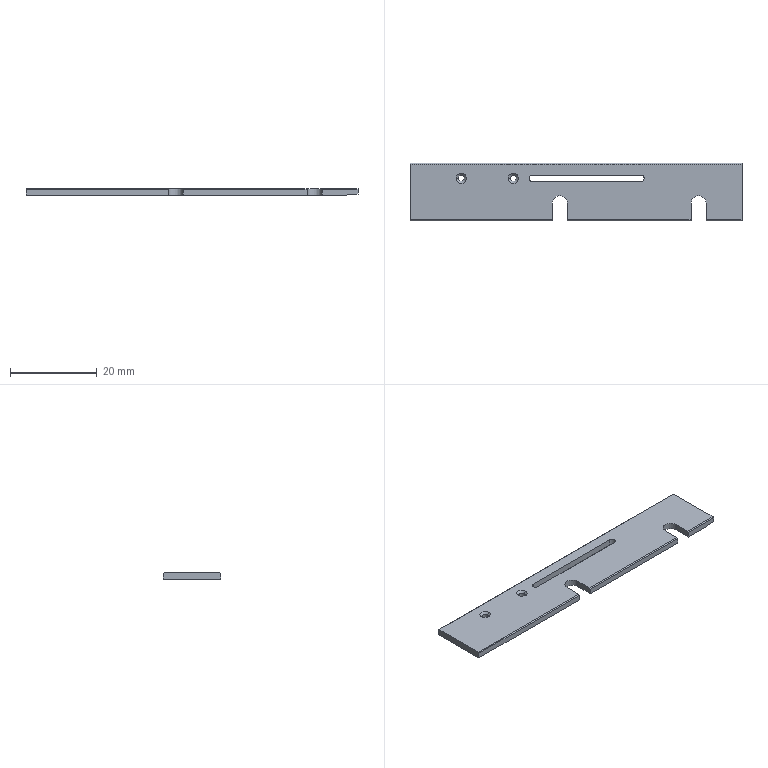Part | NX | 1 solid | 32 faces | box 76.5 x 13.2 x 1.5 mm | volume 1385 mm3 | plane 19 | cylinder 9 | cone 4 | commonest cylinder face diameters 1.4 x4 1.5 x3 3.5 x2
STEP:
#1=CARTESIAN_POINT('',(30.05,-3.5,0.75));
#2=VERTEX_POINT('',#1);
#3=CARTESIAN_POINT('',(30.05,-7.3,0.75));
#4=VERTEX_POINT('',#3);
#5=CARTESIAN_POINT('',(30.05,0.,0.75));
#6=DIRECTION('',(0.,-1.,0.));
#7=VECTOR('',#6,1000.);
#8=LINE('',#5,#7);
#9=EDGE_CURVE('',#2,#4,#8,.T.);
#10=ORIENTED_EDGE('',*,*,#9,.T.);
#11=CARTESIAN_POINT('',(38.3,-7.3,0.75));
#12=VERTEX_POINT('',#11);
#13=CARTESIAN_POINT('',(0.,-7.3,0.75));
#14=DIRECTION('',(-1.,0.,0.));
#15=VECTOR('',#14,1000.);
#16=LINE('',#13,#15);
#17=EDGE_CURVE('',#12,#4,#16,.T.);
#18=ORIENTED_EDGE('',*,*,#17,.F.);
#19=CARTESIAN_POINT('',(38.3,5.5,0.75));
#20=VERTEX_POINT('',#19);
#21=CARTESIAN_POINT('',(38.3,0.,0.75));
#22=DIRECTION('',(0.,-1.,0.));
#23=VECTOR('',#22,1000.);
#24=LINE('',#21,#23);
#25=EDGE_CURVE('',#20,#12,#24,.T.);
#26=ORIENTED_EDGE('',*,*,#25,.F.);
#27=CARTESIAN_POINT('',(-38.2,5.5,0.75));
#28=VERTEX_POINT('',#27);
#29=CARTESIAN_POINT('',(0.,5.5,0.75));
#30=DIRECTION('',(1.,0.,0.));
#31=VECTOR('',#30,1000.);
#32=LINE('',#29,#31);
#33=EDGE_CURVE('',#28,#20,#32,.T.);
#34=ORIENTED_EDGE('',*,*,#33,.F.);
#35=CARTESIAN_POINT('',(-38.2,-7.3,0.75));
#36=VERTEX_POINT('',#35);
#37=CARTESIAN_POINT('',(-38.2,0.,0.75));
#38=DIRECTION('',(0.,1.,0.));
#39=VECTOR('',#38,1000.);
#40=LINE('',#37,#39);
#41=EDGE_CURVE('',#36,#28,#40,.T.);
#42=ORIENTED_EDGE('',*,*,#41,.F.);
#43=CARTESIAN_POINT('',(-5.45,-7.3,0.75));
#44=VERTEX_POINT('',#43);
#45=CARTESIAN_POINT('',(0.,-7.3,0.75));
#46=DIRECTION('',(-1.,0.,0.));
#47=VECTOR('',#46,1000.);
#48=LINE('',#45,#47);
#49=EDGE_CURVE('',#44,#36,#48,.T.);
#50=ORIENTED_EDGE('',*,*,#49,.F.);
#51=CARTESIAN_POINT('',(-5.45,-3.5,0.75));
#52=VERTEX_POINT('',#51);
#53=CARTESIAN_POINT('',(-5.45,0.,0.75));
#54=DIRECTION('',(0.,1.,0.));
#55=VECTOR('',#54,1000.);
#56=LINE('',#53,#55);
#57=EDGE_CURVE('',#44,#52,#56,.T.);
#58=ORIENTED_EDGE('',*,*,#57,.T.);
#59=CARTESIAN_POINT('',(-1.95,-3.5,0.75));
#60=VERTEX_POINT('',#59);
#61=CARTESIAN_POINT('',(-3.7,-3.5,0.75));
#62=DIRECTION('',(0.,0.,-1.));
#63=DIRECTION('',(-1.,0.,0.));
#64=AXIS2_PLACEMENT_3D('',#61,#62,#63);
#65=CIRCLE('',#64,1.75);
#66=EDGE_CURVE('',#52,#60,#65,.T.);
#67=ORIENTED_EDGE('',*,*,#66,.T.);
#68=CARTESIAN_POINT('',(-1.95,-7.3,0.75));
#69=VERTEX_POINT('',#68);
#70=CARTESIAN_POINT('',(-1.95,0.,0.75));
#71=DIRECTION('',(0.,-1.,0.));
#72=VECTOR('',#71,1000.);
#73=LINE('',#70,#72);
#74=EDGE_CURVE('',#60,#69,#73,.T.);
#75=ORIENTED_EDGE('',*,*,#74,.T.);
#76=CARTESIAN_POINT('',(26.55,-7.3,0.75));
#77=VERTEX_POINT('',#76);
#78=CARTESIAN_POINT('',(0.,-7.3,0.75));
#79=DIRECTION('',(-1.,0.,0.));
#80=VECTOR('',#79,1000.);
#81=LINE('',#78,#80);
#82=EDGE_CURVE('',#77,#69,#81,.T.);
#83=ORIENTED_EDGE('',*,*,#82,.F.);
#84=CARTESIAN_POINT('',(26.55,-3.5,0.75));
#85=VERTEX_POINT('',#84);
#86=CARTESIAN_POINT('',(26.55,0.,0.75));
#87=DIRECTION('',(0.,1.,0.));
#88=VECTOR('',#87,1000.);
#89=LINE('',#86,#88);
#90=EDGE_CURVE('',#77,#85,#89,.T.);
#91=ORIENTED_EDGE('',*,*,#90,.T.);
#92=CARTESIAN_POINT('',(28.3,-3.5,0.75));
#93=DIRECTION('',(0.,0.,-1.));
#94=DIRECTION('',(-1.,0.,0.));
#95=AXIS2_PLACEMENT_3D('',#92,#93,#94);
#96=CIRCLE('',#95,1.75);
#97=EDGE_CURVE('',#85,#2,#96,.T.);
#98=ORIENTED_EDGE('',*,*,#97,.T.);
#99=EDGE_LOOP('',(#10,#18,#26,#34,#42,#50,#58,#67,#75,#83,#91,#98));
#100=FACE_BOUND('',#99,.T.);
#101=CARTESIAN_POINT('',(15.,1.5,0.75));
#102=VERTEX_POINT('',#101);
#103=CARTESIAN_POINT('',(15.,3.,0.75));
#104=VERTEX_POINT('',#103);
#105=CARTESIAN_POINT('',(15.,2.25,0.75));
#106=DIRECTION('',(0.,0.,1.));
#107=DIRECTION('',(-1.,0.,0.));
#108=AXIS2_PLACEMENT_3D('',#105,#106,#107);
#109=CIRCLE('',#108,0.75);
#110=EDGE_CURVE('',#102,#104,#109,.T.);
#111=ORIENTED_EDGE('',*,*,#110,.F.);
#112=CARTESIAN_POINT('',(-10.,1.5,0.75));
#113=VERTEX_POINT('',#112);
#114=CARTESIAN_POINT('',(0.,1.5,0.75));
#115=DIRECTION('',(-1.,0.,0.));
#116=VECTOR('',#115,1000.);
#117=LINE('',#114,#116);
#118=EDGE_CURVE('',#102,#113,#117,.T.);
#119=ORIENTED_EDGE('',*,*,#118,.T.);
#120=CARTESIAN_POINT('',(-10.75,2.25,0.75));
#121=VERTEX_POINT('',#120);
#122=CARTESIAN_POINT('',(-10.,2.25,0.75));
#123=DIRECTION('',(0.,0.,1.));
#124=DIRECTION('',(-1.,0.,0.));
#125=AXIS2_PLACEMENT_3D('',#122,#123,#124);
#126=CIRCLE('',#125,0.75);
#127=EDGE_CURVE('',#121,#113,#126,.T.);
#128=ORIENTED_EDGE('',*,*,#127,.F.);
#129=CARTESIAN_POINT('',(-10.,3.,0.75));
#130=VERTEX_POINT('',#129);
#131=CARTESIAN_POINT('',(-10.,2.25,0.75));
#132=DIRECTION('',(0.,0.,1.));
#133=DIRECTION('',(-1.,0.,0.));
#134=AXIS2_PLACEMENT_3D('',#131,#132,#133);
#135=CIRCLE('',#134,0.75);
#136=EDGE_CURVE('',#130,#121,#135,.T.);
#137=ORIENTED_EDGE('',*,*,#136,.F.);
#138=CARTESIAN_POINT('',(0.,3.,0.75));
#139=DIRECTION('',(1.,0.,0.));
#140=VECTOR('',#139,1000.);
#141=LINE('',#138,#140);
#142=EDGE_CURVE('',#130,#104,#141,.T.);
#143=ORIENTED_EDGE('',*,*,#142,.T.);
#144=EDGE_LOOP('',(#111,#119,#128,#137,#143));
#145=FACE_BOUND('',#144,.T.);
#146=CARTESIAN_POINT('',(-15.6,2.25,0.75));
#147=VERTEX_POINT('',#146);
#148=CARTESIAN_POINT('',(-13.2,2.25,0.75));
#149=VERTEX_POINT('',#148);
#150=CARTESIAN_POINT('',(-14.4,2.25,0.75));
#151=DIRECTION('',(0.,0.,1.));
#152=DIRECTION('',(1.,0.,0.));
#153=AXIS2_PLACEMENT_3D('',#150,#151,#152);
#154=CIRCLE('',#153,1.2);
#155=EDGE_CURVE('',#147,#149,#154,.T.);
#156=ORIENTED_EDGE('',*,*,#155,.F.);
#157=CARTESIAN_POINT('',(-14.4,2.25,0.75));
#158=DIRECTION('',(0.,0.,1.));
#159=DIRECTION('',(1.,0.,0.));
#160=AXIS2_PLACEMENT_3D('',#157,#158,#159);
#161=CIRCLE('',#160,1.2);
#162=EDGE_CURVE('',#149,#147,#161,.T.);
#163=ORIENTED_EDGE('',*,*,#162,.F.);
#164=EDGE_LOOP('',(#156,#163));
#165=FACE_BOUND('',#164,.T.);
#166=CARTESIAN_POINT('',(-25.2,2.25,0.75));
#167=VERTEX_POINT('',#166);
#168=CARTESIAN_POINT('',(-27.6,2.25,0.75));
#169=VERTEX_POINT('',#168);
#170=CARTESIAN_POINT('',(-26.4,2.25,0.75));
#171=DIRECTION('',(0.,0.,1.));
#172=DIRECTION('',(1.,0.,0.));
#173=AXIS2_PLACEMENT_3D('',#170,#171,#172);
#174=CIRCLE('',#173,1.2);
#175=EDGE_CURVE('',#167,#169,#174,.T.);
#176=ORIENTED_EDGE('',*,*,#175,.F.);
#177=CARTESIAN_POINT('',(-26.4,2.25,0.75));
#178=DIRECTION('',(0.,0.,1.));
#179=DIRECTION('',(1.,0.,0.));
#180=AXIS2_PLACEMENT_3D('',#177,#178,#179);
#181=CIRCLE('',#180,1.2);
#182=EDGE_CURVE('',#169,#167,#181,.T.);
#183=ORIENTED_EDGE('',*,*,#182,.F.);
#184=EDGE_LOOP('',(#176,#183));
#185=FACE_BOUND('',#184,.T.);
#186=CARTESIAN_POINT('',(0.,0.,0.75));
#187=DIRECTION('',(0.,0.,1.));
#188=DIRECTION('',(1.,0.,0.));
#189=AXIS2_PLACEMENT_3D('',#186,#187,#188);
#190=PLANE('',#189);
#191=ADVANCED_FACE('',(#100,#145,#165,#185),#190,.T.);
#192=CARTESIAN_POINT('',(30.05,-3.5,-0.75));
#193=VERTEX_POINT('',#192);
#194=CARTESIAN_POINT('',(30.05,-7.5,-0.75));
#195=VERTEX_POINT('',#194);
#196=CARTESIAN_POINT('',(30.05,0.,-0.75));
#197=DIRECTION('',(0.,-1.,0.));
#198=VECTOR('',#197,1000.);
#199=LINE('',#196,#198);
#200=EDGE_CURVE('',#193,#195,#199,.T.);
#201=ORIENTED_EDGE('',*,*,#200,.T.);
#202=CARTESIAN_POINT('',(30.05,-7.5,0.55));
#203=VERTEX_POINT('',#202);
#204=CARTESIAN_POINT('',(30.05,-7.5,0.75));
#205=DIRECTION('',(0.,0.,-1.));
#206=VECTOR('',#205,1000.);
#207=LINE('',#204,#206);
#208=EDGE_CURVE('',#203,#195,#207,.T.);
#209=ORIENTED_EDGE('',*,*,#208,.F.);
#210=CARTESIAN_POINT('',(30.05,0.,8.05));
#211=DIRECTION('',(0.,0.7071,0.7071));
#212=VECTOR('',#211,1000.);
#213=LINE('',#210,#212);
#214=EDGE_CURVE('',#203,#4,#213,.T.);
#215=ORIENTED_EDGE('',*,*,#214,.T.);
#216=ORIENTED_EDGE('',*,*,#9,.F.);
#217=CARTESIAN_POINT('',(30.05,-3.5,0.75));
#218=DIRECTION('',(0.,0.,-1.));
#219=VECTOR('',#218,1000.);
#220=LINE('',#217,#219);
#221=EDGE_CURVE('',#2,#193,#220,.T.);
#222=ORIENTED_EDGE('',*,*,#221,.T.);
#223=EDGE_LOOP('',(#201,#209,#215,#216,#222));
#224=FACE_BOUND('',#223,.T.);
#225=CARTESIAN_POINT('',(30.05,-7.5,0.75));
#226=DIRECTION('',(1.,0.,0.));
#227=DIRECTION('',(0.,1.,0.));
#228=AXIS2_PLACEMENT_3D('',#225,#226,#227);
#229=PLANE('',#228);
#230=ADVANCED_FACE('',(#224),#229,.F.);
#231=ORIENTED_EDGE('',*,*,#221,.F.);
#232=ORIENTED_EDGE('',*,*,#97,.F.);
#233=CARTESIAN_POINT('',(26.55,-3.5,-0.75));
#234=VERTEX_POINT('',#233);
#235=CARTESIAN_POINT('',(26.55,-3.5,0.75));
#236=DIRECTION('',(0.,0.,-1.));
#237=VECTOR('',#236,1000.);
#238=LINE('',#235,#237);
#239=EDGE_CURVE('',#85,#234,#238,.T.);
#240=ORIENTED_EDGE('',*,*,#239,.T.);
#241=CARTESIAN_POINT('',(28.3,-3.5,-0.75));
#242=DIRECTION('',(0.,0.,-1.));
#243=DIRECTION('',(-1.,0.,0.));
#244=AXIS2_PLACEMENT_3D('',#241,#242,#243);
#245=CIRCLE('',#244,1.75);
#246=EDGE_CURVE('',#234,#193,#245,.T.);
#247=ORIENTED_EDGE('',*,*,#246,.T.);
#248=EDGE_LOOP('',(#231,#232,#240,#247));
#249=FACE_BOUND('',#248,.T.);
#250=CARTESIAN_POINT('',(28.3,-3.5,0.75));
#251=DIRECTION('',(0.,0.,-1.));
#252=DIRECTION('',(-1.,0.,0.));
#253=AXIS2_PLACEMENT_3D('',#250,#251,#252);
#254=CYLINDRICAL_SURFACE('',#253,1.75);
#255=ADVANCED_FACE('',(#249),#254,.F.);
#256=CARTESIAN_POINT('',(26.55,-7.5,-0.75));
#257=VERTEX_POINT('',#256);
#258=CARTESIAN_POINT('',(26.55,0.,-0.75));
#259=DIRECTION('',(0.,1.,0.));
#260=VECTOR('',#259,1000.);
#261=LINE('',#258,#260);
#262=EDGE_CURVE('',#257,#234,#261,.T.);
#263=ORIENTED_EDGE('',*,*,#262,.T.);
#264=ORIENTED_EDGE('',*,*,#239,.F.);
#265=ORIENTED_EDGE('',*,*,#90,.F.);
#266=CARTESIAN_POINT('',(26.55,-7.5,0.55));
#267=VERTEX_POINT('',#266);
#268=CARTESIAN_POINT('',(26.55,0.,8.05));
#269=DIRECTION('',(0.,-0.7071,-0.7071));
#270=VECTOR('',#269,1000.);
#271=LINE('',#268,#270);
#272=EDGE_CURVE('',#77,#267,#271,.T.);
#273=ORIENTED_EDGE('',*,*,#272,.T.);
#274=CARTESIAN_POINT('',(26.55,-7.5,0.75));
#275=DIRECTION('',(0.,0.,-1.));
#276=VECTOR('',#275,1000.);
#277=LINE('',#274,#276);
#278=EDGE_CURVE('',#267,#257,#277,.T.);
#279=ORIENTED_EDGE('',*,*,#278,.T.);
#280=EDGE_LOOP('',(#263,#264,#265,#273,#279));
#281=FACE_BOUND('',#280,.T.);
#282=CARTESIAN_POINT('',(26.55,-3.5,0.75));
#283=DIRECTION('',(-1.,0.,0.));
#284=DIRECTION('',(0.,0.,1.));
#285=AXIS2_PLACEMENT_3D('',#282,#283,#284);
#286=PLANE('',#285);
#287=ADVANCED_FACE('',(#281),#286,.F.);
#288=CARTESIAN_POINT('',(-1.95,-7.5,0.55));
#289=VERTEX_POINT('',#288);
#290=CARTESIAN_POINT('',(0.,-7.5,0.55));
#291=DIRECTION('',(1.,0.,0.));
#292=VECTOR('',#291,1000.);
#293=LINE('',#290,#292);
#294=EDGE_CURVE('',#289,#267,#293,.T.);
#295=ORIENTED_EDGE('',*,*,#294,.F.);
#296=CARTESIAN_POINT('',(-1.95,-7.5,-0.75));
#297=VERTEX_POINT('',#296);
#298=CARTESIAN_POINT('',(-1.95,-7.5,0.75));
#299=DIRECTION('',(0.,0.,-1.));
#300=VECTOR('',#299,1000.);
#301=LINE('',#298,#300);
#302=EDGE_CURVE('',#289,#297,#301,.T.);
#303=ORIENTED_EDGE('',*,*,#302,.T.);
#304=CARTESIAN_POINT('',(0.,-7.5,-0.75));
#305=DIRECTION('',(-1.,0.,0.));
#306=VECTOR('',#305,1000.);
#307=LINE('',#304,#306);
#308=EDGE_CURVE('',#257,#297,#307,.T.);
#309=ORIENTED_EDGE('',*,*,#308,.F.);
#310=ORIENTED_EDGE('',*,*,#278,.F.);
#311=EDGE_LOOP('',(#295,#303,#309,#310));
#312=FACE_BOUND('',#311,.T.);
#313=CARTESIAN_POINT('',(-38.3,-7.5,-0.75));
#314=DIRECTION('',(0.,-1.,0.));
#315=DIRECTION('',(0.,0.,-1.));
#316=AXIS2_PLACEMENT_3D('',#313,#314,#315);
#317=PLANE('',#316);
#318=ADVANCED_FACE('',(#312),#317,.T.);
#319=CARTESIAN_POINT('',(-1.95,-3.5,-0.75));
#320=VERTEX_POINT('',#319);
#321=CARTESIAN_POINT('',(-1.95,0.,-0.75));
#322=DIRECTION('',(0.,-1.,0.));
#323=VECTOR('',#322,1000.);
#324=LINE('',#321,#323);
#325=EDGE_CURVE('',#320,#297,#324,.T.);
#326=ORIENTED_EDGE('',*,*,#325,.T.);
#327=ORIENTED_EDGE('',*,*,#302,.F.);
#328=CARTESIAN_POINT('',(-1.95,0.,8.05));
#329=DIRECTION('',(0.,0.7071,0.7071));
#330=VECTOR('',#329,1000.);
#331=LINE('',#328,#330);
#332=EDGE_CURVE('',#289,#69,#331,.T.);
#333=ORIENTED_EDGE('',*,*,#332,.T.);
#334=ORIENTED_EDGE('',*,*,#74,.F.);
#335=CARTESIAN_POINT('',(-1.95,-3.5,0.75));
#336=DIRECTION('',(0.,0.,-1.));
#337=VECTOR('',#336,1000.);
#338=LINE('',#335,#337);
#339=EDGE_CURVE('',#60,#320,#338,.T.);
#340=ORIENTED_EDGE('',*,*,#339,.T.);
#341=EDGE_LOOP('',(#326,#327,#333,#334,#340));
#342=FACE_BOUND('',#341,.T.);
#343=CARTESIAN_POINT('',(-1.95,-7.5,0.75));
#344=DIRECTION('',(1.,0.,0.));
#345=DIRECTION('',(0.,1.,0.));
#346=AXIS2_PLACEMENT_3D('',#343,#344,#345);
#347=PLANE('',#346);
#348=ADVANCED_FACE('',(#342),#347,.F.);
#349=ORIENTED_EDGE('',*,*,#339,.F.);
#350=ORIENTED_EDGE('',*,*,#66,.F.);
#351=CARTESIAN_POINT('',(-5.45,-3.5,-0.75));
#352=VERTEX_POINT('',#351);
#353=CARTESIAN_POINT('',(-5.45,-3.5,0.75));
#354=DIRECTION('',(0.,0.,-1.));
#355=VECTOR('',#354,1000.);
#356=LINE('',#353,#355);
#357=EDGE_CURVE('',#52,#352,#356,.T.);
#358=ORIENTED_EDGE('',*,*,#357,.T.);
#359=CARTESIAN_POINT('',(-3.7,-3.5,-0.75));
#360=DIRECTION('',(0.,0.,-1.));
#361=DIRECTION('',(-1.,0.,0.));
#362=AXIS2_PLACEMENT_3D('',#359,#360,#361);
#363=CIRCLE('',#362,1.75);
#364=EDGE_CURVE('',#352,#320,#363,.T.);
#365=ORIENTED_EDGE('',*,*,#364,.T.);
#366=EDGE_LOOP('',(#349,#350,#358,#365));
#367=FACE_BOUND('',#366,.T.);
#368=CARTESIAN_POINT('',(-3.7,-3.5,0.75));
#369=DIRECTION('',(0.,0.,-1.));
#370=DIRECTION('',(-1.,0.,0.));
#371=AXIS2_PLACEMENT_3D('',#368,#369,#370);
#372=CYLINDRICAL_SURFACE('',#371,1.75);
#373=ADVANCED_FACE('',(#367),#372,.F.);
#374=CARTESIAN_POINT('',(-5.45,-7.5,-0.75));
#375=VERTEX_POINT('',#374);
#376=CARTESIAN_POINT('',(-5.45,0.,-0.75));
#377=DIRECTION('',(0.,1.,0.));
#378=VECTOR('',#377,1000.);
#379=LINE('',#376,#378);
#380=EDGE_CURVE('',#375,#352,#379,.T.);
#381=ORIENTED_EDGE('',*,*,#380,.T.);
#382=ORIENTED_EDGE('',*,*,#357,.F.);
#383=ORIENTED_EDGE('',*,*,#57,.F.);
#384=CARTESIAN_POINT('',(-5.45,-7.5,0.55));
#385=VERTEX_POINT('',#384);
#386=CARTESIAN_POINT('',(-5.45,0.,8.05));
#387=DIRECTION('',(0.,0.7071,0.7071));
#388=VECTOR('',#387,1000.);
#389=LINE('',#386,#388);
#390=EDGE_CURVE('',#385,#44,#389,.T.);
#391=ORIENTED_EDGE('',*,*,#390,.F.);
#392=CARTESIAN_POINT('',(-5.45,-7.5,0.));
#393=DIRECTION('',(0.,0.,1.));
#394=VECTOR('',#393,1000.);
#395=LINE('',#392,#394);
#396=EDGE_CURVE('',#375,#385,#395,.T.);
#397=ORIENTED_EDGE('',*,*,#396,.F.);
#398=EDGE_LOOP('',(#381,#382,#383,#391,#397));
#399=FACE_BOUND('',#398,.T.);
#400=CARTESIAN_POINT('',(-5.45,-3.5,0.75));
#401=DIRECTION('',(-1.,0.,0.));
#402=DIRECTION('',(0.,0.,1.));
#403=AXIS2_PLACEMENT_3D('',#400,#401,#402);
#404=PLANE('',#403);
#405=ADVANCED_FACE('',(#399),#404,.F.);
#406=CARTESIAN_POINT('',(-38.2,-7.5,0.55));
#407=VERTEX_POINT('',#406);
#408=CARTESIAN_POINT('',(0.,-7.5,0.55));
#409=DIRECTION('',(1.,0.,0.));
#410=VECTOR('',#409,1000.);
#411=LINE('',#408,#410);
#412=EDGE_CURVE('',#407,#385,#411,.T.);
#413=ORIENTED_EDGE('',*,*,#412,.F.);
#414=CARTESIAN_POINT('',(-38.2,-7.5,-0.75));
#415=VERTEX_POINT('',#414);
#416=CARTESIAN_POINT('',(-38.2,-7.5,0.));
#417=DIRECTION('',(0.,0.,1.));
#418=VECTOR('',#417,1000.);
#419=LINE('',#416,#418);
#420=EDGE_CURVE('',#415,#407,#419,.T.);
#421=ORIENTED_EDGE('',*,*,#420,.F.);
#422=CARTESIAN_POINT('',(0.,-7.5,-0.75));
#423=DIRECTION('',(1.,0.,0.));
#424=VECTOR('',#423,1000.);
#425=LINE('',#422,#424);
#426=EDGE_CURVE('',#415,#375,#425,.T.);
#427=ORIENTED_EDGE('',*,*,#426,.T.);
#428=ORIENTED_EDGE('',*,*,#396,.T.);
#429=EDGE_LOOP('',(#413,#421,#427,#428));
#430=FACE_BOUND('',#429,.T.);
#431=CARTESIAN_POINT('',(-38.3,-7.5,-0.75));
#432=DIRECTION('',(0.,-1.,0.));
#433=DIRECTION('',(0.,0.,-1.));
#434=AXIS2_PLACEMENT_3D('',#431,#432,#433);
#435=PLANE('',#434);
#436=ADVANCED_FACE('',(#430),#435,.T.);
#437=CARTESIAN_POINT('',(-38.2,5.7,-0.75));
#438=VERTEX_POINT('',#437);
#439=CARTESIAN_POINT('',(-38.2,0.,-0.75));
#440=DIRECTION('',(0.,1.,0.));
#441=VECTOR('',#440,1000.);
#442=LINE('',#439,#441);
#443=EDGE_CURVE('',#415,#438,#442,.T.);
#444=ORIENTED_EDGE('',*,*,#443,.F.);
#445=ORIENTED_EDGE('',*,*,#420,.T.);
#446=CARTESIAN_POINT('',(-38.2,0.,8.05));
#447=DIRECTION('',(0.,0.7071,0.7071));
#448=VECTOR('',#447,1000.);
#449=LINE('',#446,#448);
#450=EDGE_CURVE('',#407,#36,#449,.T.);
#451=ORIENTED_EDGE('',*,*,#450,.T.);
#452=ORIENTED_EDGE('',*,*,#41,.T.);
#453=CARTESIAN_POINT('',(-38.2,5.7,0.55));
#454=VERTEX_POINT('',#453);
#455=CARTESIAN_POINT('',(-38.2,0.,6.25));
#456=DIRECTION('',(0.,0.7071,-0.7071));
#457=VECTOR('',#456,1000.);
#458=LINE('',#455,#457);
#459=EDGE_CURVE('',#28,#454,#458,.T.);
#460=ORIENTED_EDGE('',*,*,#459,.T.);
#461=CARTESIAN_POINT('',(-38.2,5.7,0.));
#462=DIRECTION('',(0.,0.,-1.));
#463=VECTOR('',#462,1000.);
#464=LINE('',#461,#463);
#465=EDGE_CURVE('',#454,#438,#464,.T.);
#466=ORIENTED_EDGE('',*,*,#465,.T.);
#467=EDGE_LOOP('',(#444,#445,#451,#452,#460,#466));
#468=FACE_BOUND('',#467,.T.);
#469=CARTESIAN_POINT('',(-38.2,7.5,-0.75));
#470=DIRECTION('',(-1.,0.,0.));
#471=DIRECTION('',(0.,0.,1.));
#472=AXIS2_PLACEMENT_3D('',#469,#470,#471);
#473=PLANE('',#472);
#474=ADVANCED_FACE('',(#468),#473,.T.);
#475=CARTESIAN_POINT('',(38.3,5.7,0.55));
#476=VERTEX_POINT('',#475);
#477=CARTESIAN_POINT('',(0.,5.7,0.55));
#478=DIRECTION('',(1.,0.,0.));
#479=VECTOR('',#478,1000.);
#480=LINE('',#477,#479);
#481=EDGE_CURVE('',#454,#476,#480,.T.);
#482=ORIENTED_EDGE('',*,*,#481,.T.);
#483=CARTESIAN_POINT('',(38.3,5.7,-0.4875));
#484=VERTEX_POINT('',#483);
#485=CARTESIAN_POINT('',(38.3,5.7,0.));
#486=DIRECTION('',(0.,0.,1.));
#487=VECTOR('',#486,1000.);
#488=LINE('',#485,#487);
#489=EDGE_CURVE('',#484,#476,#488,.T.);
#490=ORIENTED_EDGE('',*,*,#489,.F.);
#491=CARTESIAN_POINT('',(35.3,5.7,-0.75));
#492=VERTEX_POINT('',#491);
#493=CARTESIAN_POINT('',(0.,5.7,-3.838));
#494=DIRECTION('',(0.9962,0.,0.08716));
#495=VECTOR('',#494,1000.);
#496=LINE('',#493,#495);
#497=EDGE_CURVE('',#492,#484,#496,.T.);
#498=ORIENTED_EDGE('',*,*,#497,.F.);
#499=CARTESIAN_POINT('',(0.,5.7,-0.75));
#500=DIRECTION('',(1.,0.,0.));
#501=VECTOR('',#500,1000.);
#502=LINE('',#499,#501);
#503=EDGE_CURVE('',#438,#492,#502,.T.);
#504=ORIENTED_EDGE('',*,*,#503,.F.);
#505=ORIENTED_EDGE('',*,*,#465,.F.);
#506=EDGE_LOOP('',(#482,#490,#498,#504,#505));
#507=FACE_BOUND('',#506,.T.);
#508=CARTESIAN_POINT('',(38.3,5.7,-0.75));
#509=DIRECTION('',(0.,1.,0.));
#510=DIRECTION('',(1.,0.,0.));
#511=AXIS2_PLACEMENT_3D('',#508,#509,#510);
#512=PLANE('',#511);
#513=ADVANCED_FACE('',(#507),#512,.T.);
#514=CARTESIAN_POINT('',(35.3,-7.5,-0.75));
#515=VERTEX_POINT('',#514);
#516=CARTESIAN_POINT('',(35.3,0.,-0.75));
#517=DIRECTION('',(0.,-1.,0.));
#518=VECTOR('',#517,1000.);
#519=LINE('',#516,#518);
#520=EDGE_CURVE('',#492,#515,#519,.T.);
#521=ORIENTED_EDGE('',*,*,#520,.F.);
#522=ORIENTED_EDGE('',*,*,#497,.T.);
#523=CARTESIAN_POINT('',(38.3,-7.5,-0.4875));
#524=VERTEX_POINT('',#523);
#525=CARTESIAN_POINT('',(38.3,0.,-0.4875));
#526=DIRECTION('',(0.,-1.,0.));
#527=VECTOR('',#526,1000.);
#528=LINE('',#525,#527);
#529=EDGE_CURVE('',#484,#524,#528,.T.);
#530=ORIENTED_EDGE('',*,*,#529,.T.);
#531=CARTESIAN_POINT('',(0.,-7.5,-3.838));
#532=DIRECTION('',(0.9962,0.,0.08716));
#533=VECTOR('',#532,1000.);
#534=LINE('',#531,#533);
#535=EDGE_CURVE('',#515,#524,#534,.T.);
#536=ORIENTED_EDGE('',*,*,#535,.F.);
#537=EDGE_LOOP('',(#521,#522,#530,#536));
#538=FACE_BOUND('',#537,.T.);
#539=CARTESIAN_POINT('',(35.3,-7.5,-0.75));
#540=DIRECTION('',(0.08716,0.,-0.9962));
#541=DIRECTION('',(0.,-1.,0.));
#542=AXIS2_PLACEMENT_3D('',#539,#540,#541);
#543=PLANE('',#542);
#544=ADVANCED_FACE('',(#538),#543,.T.);
#545=CARTESIAN_POINT('',(38.3,-7.5,0.55));
#546=VERTEX_POINT('',#545);
#547=CARTESIAN_POINT('',(0.,-7.5,0.55));
#548=DIRECTION('',(1.,0.,0.));
#549=VECTOR('',#548,1000.);
#550=LINE('',#547,#549);
#551=EDGE_CURVE('',#203,#546,#550,.T.);
#552=ORIENTED_EDGE('',*,*,#551,.F.);
#553=ORIENTED_EDGE('',*,*,#208,.T.);
#554=CARTESIAN_POINT('',(0.,-7.5,-0.75));
#555=DIRECTION('',(-1.,0.,0.));
#556=VECTOR('',#555,1000.);
#557=LINE('',#554,#556);
#558=EDGE_CURVE('',#515,#195,#557,.T.);
#559=ORIENTED_EDGE('',*,*,#558,.F.);
#560=ORIENTED_EDGE('',*,*,#535,.T.);
#561=CARTESIAN_POINT('',(38.3,-7.5,0.));
#562=DIRECTION('',(0.,0.,1.));
#563=VECTOR('',#562,1000.);
#564=LINE('',#561,#563);
#565=EDGE_CURVE('',#524,#546,#564,.T.);
#566=ORIENTED_EDGE('',*,*,#565,.T.);
#567=EDGE_LOOP('',(#552,#553,#559,#560,#566));
#568=FACE_BOUND('',#567,.T.);
#569=CARTESIAN_POINT('',(-38.3,-7.5,-0.75));
#570=DIRECTION('',(0.,-1.,0.));
#571=DIRECTION('',(0.,0.,-1.));
#572=AXIS2_PLACEMENT_3D('',#569,#570,#571);
#573=PLANE('',#572);
#574=ADVANCED_FACE('',(#568),#573,.T.);
#575=ORIENTED_EDGE('',*,*,#200,.F.);
#576=ORIENTED_EDGE('',*,*,#246,.F.);
#577=ORIENTED_EDGE('',*,*,#262,.F.);
#578=ORIENTED_EDGE('',*,*,#308,.T.);
#579=ORIENTED_EDGE('',*,*,#325,.F.);
#580=ORIENTED_EDGE('',*,*,#364,.F.);
#581=ORIENTED_EDGE('',*,*,#380,.F.);
#582=ORIENTED_EDGE('',*,*,#426,.F.);
#583=ORIENTED_EDGE('',*,*,#443,.T.);
#584=ORIENTED_EDGE('',*,*,#503,.T.);
#585=ORIENTED_EDGE('',*,*,#520,.T.);
#586=ORIENTED_EDGE('',*,*,#558,.T.);
#587=EDGE_LOOP('',(#575,#576,#577,#578,#579,#580,#581,#582,#583,#584,#585,#586));
#588=FACE_BOUND('',#587,.T.);
#589=CARTESIAN_POINT('',(-13.7,2.25,-0.75));
#590=VERTEX_POINT('',#589);
#591=CARTESIAN_POINT('',(-15.1,2.25,-0.75));
#592=VERTEX_POINT('',#591);
#593=CARTESIAN_POINT('',(-14.4,2.25,-0.75));
#594=DIRECTION('',(0.,0.,1.));
#595=DIRECTION('',(1.,0.,0.));
#596=AXIS2_PLACEMENT_3D('',#593,#594,#595);
#597=CIRCLE('',#596,0.7);
#598=EDGE_CURVE('',#590,#592,#597,.T.);
#599=ORIENTED_EDGE('',*,*,#598,.T.);
#600=CARTESIAN_POINT('',(-14.4,2.25,-0.75));
#601=DIRECTION('',(0.,0.,1.));
#602=DIRECTION('',(1.,0.,0.));
#603=AXIS2_PLACEMENT_3D('',#600,#601,#602);
#604=CIRCLE('',#603,0.7);
#605=EDGE_CURVE('',#592,#590,#604,.T.);
#606=ORIENTED_EDGE('',*,*,#605,.T.);
#607=EDGE_LOOP('',(#599,#606));
#608=FACE_BOUND('',#607,.T.);
#609=CARTESIAN_POINT('',(-27.1,2.25,-0.75));
#610=VERTEX_POINT('',#609);
#611=CARTESIAN_POINT('',(-25.7,2.25,-0.75));
#612=VERTEX_POINT('',#611);
#613=CARTESIAN_POINT('',(-26.4,2.25,-0.75));
#614=DIRECTION('',(0.,0.,1.));
#615=DIRECTION('',(1.,0.,0.));
#616=AXIS2_PLACEMENT_3D('',#613,#614,#615);
#617=CIRCLE('',#616,0.7);
#618=EDGE_CURVE('',#610,#612,#617,.T.);
#619=ORIENTED_EDGE('',*,*,#618,.T.);
#620=CARTESIAN_POINT('',(-26.4,2.25,-0.75));
#621=DIRECTION('',(0.,0.,1.));
#622=DIRECTION('',(1.,0.,0.));
#623=AXIS2_PLACEMENT_3D('',#620,#621,#622);
#624=CIRCLE('',#623,0.7);
#625=EDGE_CURVE('',#612,#610,#624,.T.);
#626=ORIENTED_EDGE('',*,*,#625,.T.);
#627=EDGE_LOOP('',(#619,#626));
#628=FACE_BOUND('',#627,.T.);
#629=CARTESIAN_POINT('',(15.,1.5,-0.75));
#630=VERTEX_POINT('',#629);
#631=CARTESIAN_POINT('',(15.,3.,-0.75));
#632=VERTEX_POINT('',#631);
#633=CARTESIAN_POINT('',(15.,2.25,-0.75));
#634=DIRECTION('',(0.,0.,1.));
#635=DIRECTION('',(-1.,0.,0.));
#636=AXIS2_PLACEMENT_3D('',#633,#634,#635);
#637=CIRCLE('',#636,0.75);
#638=EDGE_CURVE('',#630,#632,#637,.T.);
#639=ORIENTED_EDGE('',*,*,#638,.T.);
#640=CARTESIAN_POINT('',(-10.,3.,-0.75));
#641=VERTEX_POINT('',#640);
#642=CARTESIAN_POINT('',(0.,3.,-0.75));
#643=DIRECTION('',(1.,0.,0.));
#644=VECTOR('',#643,1000.);
#645=LINE('',#642,#644);
#646=EDGE_CURVE('',#641,#632,#645,.T.);
#647=ORIENTED_EDGE('',*,*,#646,.F.);
#648=CARTESIAN_POINT('',(-10.75,2.25,-0.75));
#649=VERTEX_POINT('',#648);
#650=CARTESIAN_POINT('',(-10.,2.25,-0.75));
#651=DIRECTION('',(0.,0.,1.));
#652=DIRECTION('',(-1.,0.,0.));
#653=AXIS2_PLACEMENT_3D('',#650,#651,#652);
#654=CIRCLE('',#653,0.75);
#655=EDGE_CURVE('',#641,#649,#654,.T.);
#656=ORIENTED_EDGE('',*,*,#655,.T.);
#657=CARTESIAN_POINT('',(-10.,1.5,-0.75));
#658=VERTEX_POINT('',#657);
#659=CARTESIAN_POINT('',(-10.,2.25,-0.75));
#660=DIRECTION('',(0.,0.,1.));
#661=DIRECTION('',(-1.,0.,0.));
#662=AXIS2_PLACEMENT_3D('',#659,#660,#661);
#663=CIRCLE('',#662,0.75);
#664=EDGE_CURVE('',#649,#658,#663,.T.);
#665=ORIENTED_EDGE('',*,*,#664,.T.);
#666=CARTESIAN_POINT('',(0.,1.5,-0.75));
#667=DIRECTION('',(-1.,0.,0.));
#668=VECTOR('',#667,1000.);
#669=LINE('',#666,#668);
#670=EDGE_CURVE('',#630,#658,#669,.T.);
#671=ORIENTED_EDGE('',*,*,#670,.F.);
#672=EDGE_LOOP('',(#639,#647,#656,#665,#671));
#673=FACE_BOUND('',#672,.T.);
#674=CARTESIAN_POINT('',(0.,0.,-0.75));
#675=DIRECTION('',(0.,0.,1.));
#676=DIRECTION('',(1.,0.,0.));
#677=AXIS2_PLACEMENT_3D('',#674,#675,#676);
#678=PLANE('',#677);
#679=ADVANCED_FACE('',(#588,#608,#628,#673),#678,.F.);
#680=ORIENTED_EDGE('',*,*,#529,.F.);
#681=ORIENTED_EDGE('',*,*,#489,.T.);
#682=CARTESIAN_POINT('',(38.3,0.,6.25));
#683=DIRECTION('',(0.,-0.7071,0.7071));
#684=VECTOR('',#683,1000.);
#685=LINE('',#682,#684);
#686=EDGE_CURVE('',#476,#20,#685,.T.);
#687=ORIENTED_EDGE('',*,*,#686,.T.);
#688=ORIENTED_EDGE('',*,*,#25,.T.);
#689=CARTESIAN_POINT('',(38.3,0.,8.05));
#690=DIRECTION('',(0.,0.7071,0.7071));
#691=VECTOR('',#690,1000.);
#692=LINE('',#689,#691);
#693=EDGE_CURVE('',#546,#12,#692,.T.);
#694=ORIENTED_EDGE('',*,*,#693,.F.);
#695=ORIENTED_EDGE('',*,*,#565,.F.);
#696=EDGE_LOOP('',(#680,#681,#687,#688,#694,#695));
#697=FACE_BOUND('',#696,.T.);
#698=CARTESIAN_POINT('',(38.3,-7.5,-0.75));
#699=DIRECTION('',(1.,0.,0.));
#700=DIRECTION('',(0.,1.,0.));
#701=AXIS2_PLACEMENT_3D('',#698,#699,#700);
#702=PLANE('',#701);
#703=ADVANCED_FACE('',(#697),#702,.T.);
#704=ORIENTED_EDGE('',*,*,#551,.T.);
#705=ORIENTED_EDGE('',*,*,#693,.T.);
#706=ORIENTED_EDGE('',*,*,#17,.T.);
#707=ORIENTED_EDGE('',*,*,#214,.F.);
#708=EDGE_LOOP('',(#704,#705,#706,#707));
#709=FACE_BOUND('',#708,.T.);
#710=CARTESIAN_POINT('',(34.175,-7.4,0.65));
#711=DIRECTION('',(0.,-0.7071,0.7071));
#712=DIRECTION('',(-1.,0.,0.));
#713=AXIS2_PLACEMENT_3D('',#710,#711,#712);
#714=PLANE('',#713);
#715=ADVANCED_FACE('',(#709),#714,.T.);
#716=CARTESIAN_POINT('',(-10.75,2.25,0.75));
#717=DIRECTION('',(0.,0.,1.));
#718=VECTOR('',#717,1000.);
#719=LINE('',#716,#718);
#720=EDGE_CURVE('',#649,#121,#719,.T.);
#721=ORIENTED_EDGE('',*,*,#720,.F.);
#722=ORIENTED_EDGE('',*,*,#655,.F.);
#723=CARTESIAN_POINT('',(-10.,3.,0.75));
#724=DIRECTION('',(0.,0.,-1.));
#725=VECTOR('',#724,1000.);
#726=LINE('',#723,#725);
#727=EDGE_CURVE('',#130,#641,#726,.T.);
#728=ORIENTED_EDGE('',*,*,#727,.F.);
#729=ORIENTED_EDGE('',*,*,#136,.T.);
#730=EDGE_LOOP('',(#721,#722,#728,#729));
#731=FACE_BOUND('',#730,.T.);
#732=CARTESIAN_POINT('',(-10.,2.25,0.75));
#733=DIRECTION('',(0.,0.,1.));
#734=DIRECTION('',(-1.,0.,0.));
#735=AXIS2_PLACEMENT_3D('',#732,#733,#734);
#736=CYLINDRICAL_SURFACE('',#735,0.75);
#737=ADVANCED_FACE('',(#731),#736,.F.);
#738=CARTESIAN_POINT('',(-13.7,2.25,0.25));
#739=VERTEX_POINT('',#738);
#740=CARTESIAN_POINT('',(-15.1,2.25,0.25));
#741=VERTEX_POINT('',#740);
#742=CARTESIAN_POINT('',(-14.4,2.25,0.25));
#743=DIRECTION('',(0.,0.,1.));
#744=DIRECTION('',(1.,0.,0.));
#745=AXIS2_PLACEMENT_3D('',#742,#743,#744);
#746=CIRCLE('',#745,0.7);
#747=EDGE_CURVE('',#739,#741,#746,.T.);
#748=ORIENTED_EDGE('',*,*,#747,.T.);
#749=CARTESIAN_POINT('',(-15.1,2.25,-0.75));
#750=DIRECTION('',(0.,0.,1.));
#751=VECTOR('',#750,1000.);
#752=LINE('',#749,#751);
#753=EDGE_CURVE('',#592,#741,#752,.T.);
#754=ORIENTED_EDGE('',*,*,#753,.F.);
#755=ORIENTED_EDGE('',*,*,#598,.F.);
#756=CARTESIAN_POINT('',(-13.7,2.25,-0.75));
#757=DIRECTION('',(0.,0.,1.));
#758=VECTOR('',#757,1000.);
#759=LINE('',#756,#758);
#760=EDGE_CURVE('',#590,#739,#759,.T.);
#761=ORIENTED_EDGE('',*,*,#760,.T.);
#762=EDGE_LOOP('',(#748,#754,#755,#761));
#763=FACE_BOUND('',#762,.T.);
#764=CARTESIAN_POINT('',(-14.4,2.25,-0.75));
#765=DIRECTION('',(0.,0.,1.));
#766=DIRECTION('',(1.,0.,0.));
#767=AXIS2_PLACEMENT_3D('',#764,#765,#766);
#768=CYLINDRICAL_SURFACE('',#767,0.7);
#769=ADVANCED_FACE('',(#763),#768,.F.);
#770=ORIENTED_EDGE('',*,*,#638,.F.);
#771=CARTESIAN_POINT('',(15.,1.5,0.75));
#772=DIRECTION('',(0.,0.,-1.));
#773=VECTOR('',#772,1000.);
#774=LINE('',#771,#773);
#775=EDGE_CURVE('',#102,#630,#774,.T.);
#776=ORIENTED_EDGE('',*,*,#775,.F.);
#777=ORIENTED_EDGE('',*,*,#110,.T.);
#778=CARTESIAN_POINT('',(15.,3.,-0.75));
#779=DIRECTION('',(0.,0.,1.));
#780=VECTOR('',#779,1000.);
#781=LINE('',#778,#780);
#782=EDGE_CURVE('',#632,#104,#781,.T.);
#783=ORIENTED_EDGE('',*,*,#782,.F.);
#784=EDGE_LOOP('',(#770,#776,#777,#783));
#785=FACE_BOUND('',#784,.T.);
#786=CARTESIAN_POINT('',(15.,2.25,0.75));
#787=DIRECTION('',(0.,0.,1.));
#788=DIRECTION('',(-1.,0.,0.));
#789=AXIS2_PLACEMENT_3D('',#786,#787,#788);
#790=CYLINDRICAL_SURFACE('',#789,0.75);
#791=ADVANCED_FACE('',(#785),#790,.F.);
#792=ORIENTED_EDGE('',*,*,#412,.T.);
#793=ORIENTED_EDGE('',*,*,#390,.T.);
#794=ORIENTED_EDGE('',*,*,#49,.T.);
#795=ORIENTED_EDGE('',*,*,#450,.F.);
#796=EDGE_LOOP('',(#792,#793,#794,#795));
#797=FACE_BOUND('',#796,.T.);
#798=CARTESIAN_POINT('',(-21.875,-7.4,0.65));
#799=DIRECTION('',(0.,-0.7071,0.7071));
#800=DIRECTION('',(-1.,0.,0.));
#801=AXIS2_PLACEMENT_3D('',#798,#799,#800);
#802=PLANE('',#801);
#803=ADVANCED_FACE('',(#797),#802,.T.);
#804=ORIENTED_EDGE('',*,*,#670,.T.);
#805=CARTESIAN_POINT('',(-10.,1.5,-0.75));
#806=DIRECTION('',(0.,0.,1.));
#807=VECTOR('',#806,1000.);
#808=LINE('',#805,#807);
#809=EDGE_CURVE('',#658,#113,#808,.T.);
#810=ORIENTED_EDGE('',*,*,#809,.T.);
#811=ORIENTED_EDGE('',*,*,#118,.F.);
#812=ORIENTED_EDGE('',*,*,#775,.T.);
#813=EDGE_LOOP('',(#804,#810,#811,#812));
#814=FACE_BOUND('',#813,.T.);
#815=CARTESIAN_POINT('',(-8.,1.5,0.75));
#816=DIRECTION('',(0.,-1.,0.));
#817=DIRECTION('',(0.,0.,-1.));
#818=AXIS2_PLACEMENT_3D('',#815,#816,#817);
#819=PLANE('',#818);
#820=ADVANCED_FACE('',(#814),#819,.F.);
#821=CARTESIAN_POINT('',(-27.1,2.25,0.25));
#822=VERTEX_POINT('',#821);
#823=CARTESIAN_POINT('',(-25.7,2.25,0.25));
#824=VERTEX_POINT('',#823);
#825=CARTESIAN_POINT('',(-26.4,2.25,0.25));
#826=DIRECTION('',(0.,0.,1.));
#827=DIRECTION('',(1.,0.,0.));
#828=AXIS2_PLACEMENT_3D('',#825,#826,#827);
#829=CIRCLE('',#828,0.7);
#830=EDGE_CURVE('',#822,#824,#829,.T.);
#831=ORIENTED_EDGE('',*,*,#830,.T.);
#832=CARTESIAN_POINT('',(-25.7,2.25,-0.75));
#833=DIRECTION('',(0.,0.,1.));
#834=VECTOR('',#833,1000.);
#835=LINE('',#832,#834);
#836=EDGE_CURVE('',#612,#824,#835,.T.);
#837=ORIENTED_EDGE('',*,*,#836,.F.);
#838=ORIENTED_EDGE('',*,*,#618,.F.);
#839=CARTESIAN_POINT('',(-27.1,2.25,-0.75));
#840=DIRECTION('',(0.,0.,1.));
#841=VECTOR('',#840,1000.);
#842=LINE('',#839,#841);
#843=EDGE_CURVE('',#610,#822,#842,.T.);
#844=ORIENTED_EDGE('',*,*,#843,.T.);
#845=EDGE_LOOP('',(#831,#837,#838,#844));
#846=FACE_BOUND('',#845,.T.);
#847=CARTESIAN_POINT('',(-26.4,2.25,-0.75));
#848=DIRECTION('',(0.,0.,1.));
#849=DIRECTION('',(1.,0.,0.));
#850=AXIS2_PLACEMENT_3D('',#847,#848,#849);
#851=CYLINDRICAL_SURFACE('',#850,0.7);
#852=ADVANCED_FACE('',(#846),#851,.F.);
#853=ORIENTED_EDGE('',*,*,#646,.T.);
#854=ORIENTED_EDGE('',*,*,#782,.T.);
#855=ORIENTED_EDGE('',*,*,#142,.F.);
#856=ORIENTED_EDGE('',*,*,#727,.T.);
#857=EDGE_LOOP('',(#853,#854,#855,#856));
#858=FACE_BOUND('',#857,.T.);
#859=CARTESIAN_POINT('',(15.,3.,0.75));
#860=DIRECTION('',(0.,1.,0.));
#861=DIRECTION('',(1.,0.,0.));
#862=AXIS2_PLACEMENT_3D('',#859,#860,#861);
#863=PLANE('',#862);
#864=ADVANCED_FACE('',(#858),#863,.F.);
#865=ORIENTED_EDGE('',*,*,#481,.F.);
#866=ORIENTED_EDGE('',*,*,#459,.F.);
#867=ORIENTED_EDGE('',*,*,#33,.T.);
#868=ORIENTED_EDGE('',*,*,#686,.F.);
#869=EDGE_LOOP('',(#865,#866,#867,#868));
#870=FACE_BOUND('',#869,.T.);
#871=CARTESIAN_POINT('',(0.,5.6,0.65));
#872=DIRECTION('',(0.,0.7071,0.7071));
#873=DIRECTION('',(1.,0.,0.));
#874=AXIS2_PLACEMENT_3D('',#871,#872,#873);
#875=PLANE('',#874);
#876=ADVANCED_FACE('',(#870),#875,.T.);
#877=ORIENTED_EDGE('',*,*,#294,.T.);
#878=ORIENTED_EDGE('',*,*,#272,.F.);
#879=ORIENTED_EDGE('',*,*,#82,.T.);
#880=ORIENTED_EDGE('',*,*,#332,.F.);
#881=EDGE_LOOP('',(#877,#878,#879,#880));
#882=FACE_BOUND('',#881,.T.);
#883=CARTESIAN_POINT('',(12.3,-7.4,0.65));
#884=DIRECTION('',(0.,-0.7071,0.7071));
#885=DIRECTION('',(-1.,0.,0.));
#886=AXIS2_PLACEMENT_3D('',#883,#884,#885);
#887=PLANE('',#886);
#888=ADVANCED_FACE('',(#882),#887,.T.);
#889=ORIENTED_EDGE('',*,*,#175,.T.);
#890=CARTESIAN_POINT('',(-27.1,2.25,0.25));
#891=DIRECTION('',(-0.7071,0.,0.7071));
#892=VECTOR('',#891,1000.);
#893=LINE('',#890,#892);
#894=EDGE_CURVE('',#169,#822,#893,.F.);
#895=ORIENTED_EDGE('',*,*,#894,.T.);
#896=CARTESIAN_POINT('',(-26.4,2.25,0.25));
#897=DIRECTION('',(0.,0.,1.));
#898=DIRECTION('',(1.,0.,0.));
#899=AXIS2_PLACEMENT_3D('',#896,#897,#898);
#900=CIRCLE('',#899,0.7);
#901=EDGE_CURVE('',#824,#822,#900,.T.);
#902=ORIENTED_EDGE('',*,*,#901,.F.);
#903=CARTESIAN_POINT('',(-25.7,2.25,0.25));
#904=DIRECTION('',(0.7071,0.,0.7071));
#905=VECTOR('',#904,1000.);
#906=LINE('',#903,#905);
#907=EDGE_CURVE('',#167,#824,#906,.F.);
#908=ORIENTED_EDGE('',*,*,#907,.F.);
#909=EDGE_LOOP('',(#889,#895,#902,#908));
#910=FACE_BOUND('',#909,.T.);
#911=CARTESIAN_POINT('',(-26.4,2.25,0.25));
#912=DIRECTION('',(0.,0.,1.));
#913=DIRECTION('',(1.,0.,0.));
#914=AXIS2_PLACEMENT_3D('',#911,#912,#913);
#915=CONICAL_SURFACE('',#914,0.7,0.7854);
#916=ADVANCED_FACE('',(#910),#915,.F.);
#917=ORIENTED_EDGE('',*,*,#155,.T.);
#918=CARTESIAN_POINT('',(-13.7,2.25,0.25));
#919=DIRECTION('',(0.7071,0.,0.7071));
#920=VECTOR('',#919,1000.);
#921=LINE('',#918,#920);
#922=EDGE_CURVE('',#739,#149,#921,.T.);
#923=ORIENTED_EDGE('',*,*,#922,.F.);
#924=CARTESIAN_POINT('',(-14.4,2.25,0.25));
#925=DIRECTION('',(0.,0.,1.));
#926=DIRECTION('',(1.,0.,0.));
#927=AXIS2_PLACEMENT_3D('',#924,#925,#926);
#928=CIRCLE('',#927,0.7);
#929=EDGE_CURVE('',#741,#739,#928,.T.);
#930=ORIENTED_EDGE('',*,*,#929,.F.);
#931=CARTESIAN_POINT('',(-15.1,2.25,0.25));
#932=DIRECTION('',(-0.7071,0.,0.7071));
#933=VECTOR('',#932,1000.);
#934=LINE('',#931,#933);
#935=EDGE_CURVE('',#741,#147,#934,.T.);
#936=ORIENTED_EDGE('',*,*,#935,.T.);
#937=EDGE_LOOP('',(#917,#923,#930,#936));
#938=FACE_BOUND('',#937,.T.);
#939=CARTESIAN_POINT('',(-14.4,2.25,0.25));
#940=DIRECTION('',(0.,0.,1.));
#941=DIRECTION('',(1.,0.,0.));
#942=AXIS2_PLACEMENT_3D('',#939,#940,#941);
#943=CONICAL_SURFACE('',#942,0.7,0.7854);
#944=ADVANCED_FACE('',(#938),#943,.F.);
#945=ORIENTED_EDGE('',*,*,#830,.F.);
#946=ORIENTED_EDGE('',*,*,#894,.F.);
#947=ORIENTED_EDGE('',*,*,#182,.T.);
#948=ORIENTED_EDGE('',*,*,#907,.T.);
#949=EDGE_LOOP('',(#945,#946,#947,#948));
#950=FACE_BOUND('',#949,.T.);
#951=CARTESIAN_POINT('',(-26.4,2.25,0.25));
#952=DIRECTION('',(0.,0.,1.));
#953=DIRECTION('',(1.,0.,0.));
#954=AXIS2_PLACEMENT_3D('',#951,#952,#953);
#955=CONICAL_SURFACE('',#954,0.7,0.7854);
#956=ADVANCED_FACE('',(#950),#955,.F.);
#957=ORIENTED_EDGE('',*,*,#836,.T.);
#958=ORIENTED_EDGE('',*,*,#901,.T.);
#959=ORIENTED_EDGE('',*,*,#843,.F.);
#960=ORIENTED_EDGE('',*,*,#625,.F.);
#961=EDGE_LOOP('',(#957,#958,#959,#960));
#962=FACE_BOUND('',#961,.T.);
#963=CARTESIAN_POINT('',(-26.4,2.25,-0.75));
#964=DIRECTION('',(0.,0.,1.));
#965=DIRECTION('',(1.,0.,0.));
#966=AXIS2_PLACEMENT_3D('',#963,#964,#965);
#967=CYLINDRICAL_SURFACE('',#966,0.7);
#968=ADVANCED_FACE('',(#962),#967,.F.);
#969=ORIENTED_EDGE('',*,*,#747,.F.);
#970=ORIENTED_EDGE('',*,*,#922,.T.);
#971=ORIENTED_EDGE('',*,*,#162,.T.);
#972=ORIENTED_EDGE('',*,*,#935,.F.);
#973=EDGE_LOOP('',(#969,#970,#971,#972));
#974=FACE_BOUND('',#973,.T.);
#975=CARTESIAN_POINT('',(-14.4,2.25,0.25));
#976=DIRECTION('',(0.,0.,1.));
#977=DIRECTION('',(1.,0.,0.));
#978=AXIS2_PLACEMENT_3D('',#975,#976,#977);
#979=CONICAL_SURFACE('',#978,0.7,0.7854);
#980=ADVANCED_FACE('',(#974),#979,.F.);
#981=ORIENTED_EDGE('',*,*,#760,.F.);
#982=ORIENTED_EDGE('',*,*,#605,.F.);
#983=ORIENTED_EDGE('',*,*,#753,.T.);
#984=ORIENTED_EDGE('',*,*,#929,.T.);
#985=EDGE_LOOP('',(#981,#982,#983,#984));
#986=FACE_BOUND('',#985,.T.);
#987=CARTESIAN_POINT('',(-14.4,2.25,-0.75));
#988=DIRECTION('',(0.,0.,1.));
#989=DIRECTION('',(1.,0.,0.));
#990=AXIS2_PLACEMENT_3D('',#987,#988,#989);
#991=CYLINDRICAL_SURFACE('',#990,0.7);
#992=ADVANCED_FACE('',(#986),#991,.F.);
#993=ORIENTED_EDGE('',*,*,#664,.F.);
#994=ORIENTED_EDGE('',*,*,#720,.T.);
#995=ORIENTED_EDGE('',*,*,#127,.T.);
#996=ORIENTED_EDGE('',*,*,#809,.F.);
#997=EDGE_LOOP('',(#993,#994,#995,#996));
#998=FACE_BOUND('',#997,.T.);
#999=CARTESIAN_POINT('',(-10.,2.25,0.75));
#1000=DIRECTION('',(0.,0.,1.));
#1001=DIRECTION('',(-1.,0.,0.));
#1002=AXIS2_PLACEMENT_3D('',#999,#1000,#1001);
#1003=CYLINDRICAL_SURFACE('',#1002,0.75);
#1004=ADVANCED_FACE('',(#998),#1003,.F.);
#1005=CLOSED_SHELL('',(#191,#230,#255,#287,#318,#348,#373,#405,#436,#474,#513,#544,#574,#679,#703,#715,#737,#769,#791,#803,#820,#852,#864,#876,#888,#916,#944,#956,#968,#980,#992,#1004));
#1006=MANIFOLD_SOLID_BREP('',#1005);
#1007=(LENGTH_UNIT()NAMED_UNIT(*)SI_UNIT(.MILLI.,.METRE.));
#1008=UNCERTAINTY_MEASURE_WITH_UNIT(LENGTH_MEASURE(0.00001),#1007,'','');
#1009=(NAMED_UNIT(*)PLANE_ANGLE_UNIT()SI_UNIT($,.RADIAN.));
#1010=(NAMED_UNIT(*)SI_UNIT($,.STERADIAN.)SOLID_ANGLE_UNIT());
#1011=(GEOMETRIC_REPRESENTATION_CONTEXT(3)GLOBAL_UNCERTAINTY_ASSIGNED_CONTEXT((#1008))GLOBAL_UNIT_ASSIGNED_CONTEXT((#1007,#1009,#1010))REPRESENTATION_CONTEXT('',''));
#1012=ADVANCED_BREP_SHAPE_REPRESENTATION('',(#1006),#1011);